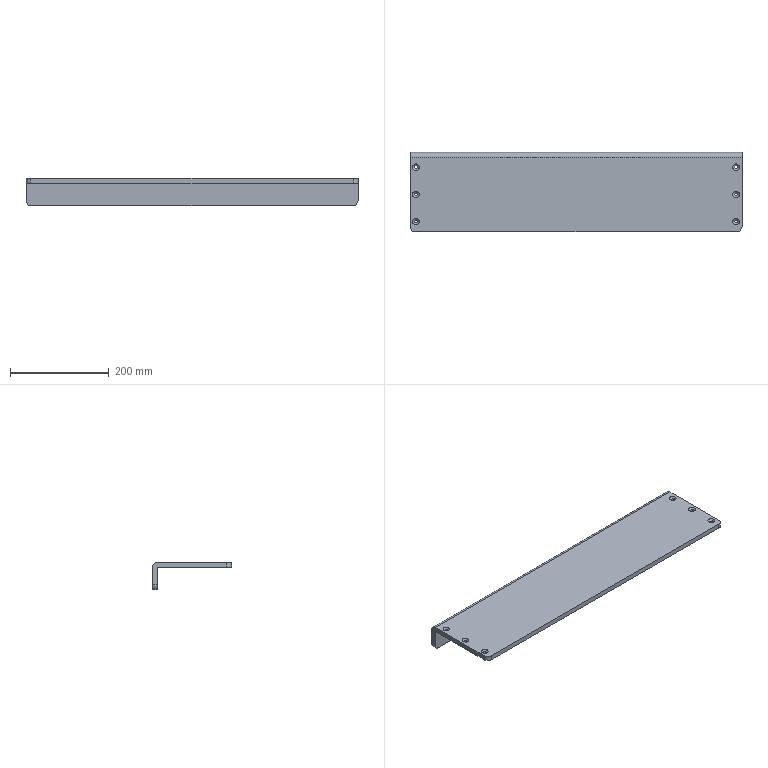Part | STEP file | QA-AD16 | 1 solid | 37 faces | box 672 x 160 x 55 mm | volume 1359289 mm3 | cylinder 17 | cone 12 | plane 8 | commonest cylinder face diameters 6.6 x12 20 x5